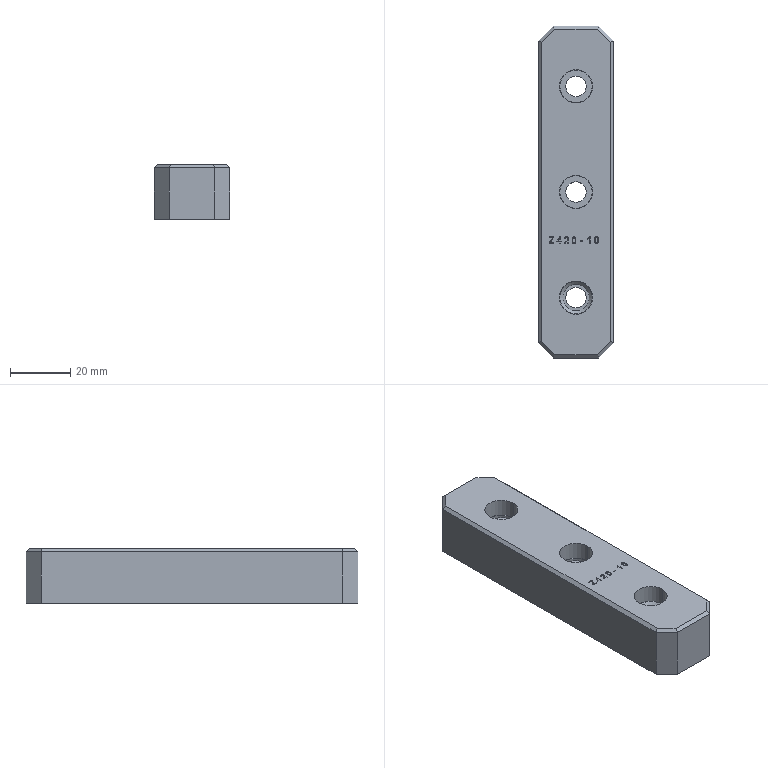Part | Creo | 1 solid | 153 faces | box 25 x 110 x 18 mm | volume 45303 mm3 | other 67 | plane 66 | cylinder 18 | cone 2 | commonest cylinder face diameters 6.8 x6 11 x6 10.8 x4 1.927 x1 30.388 x1